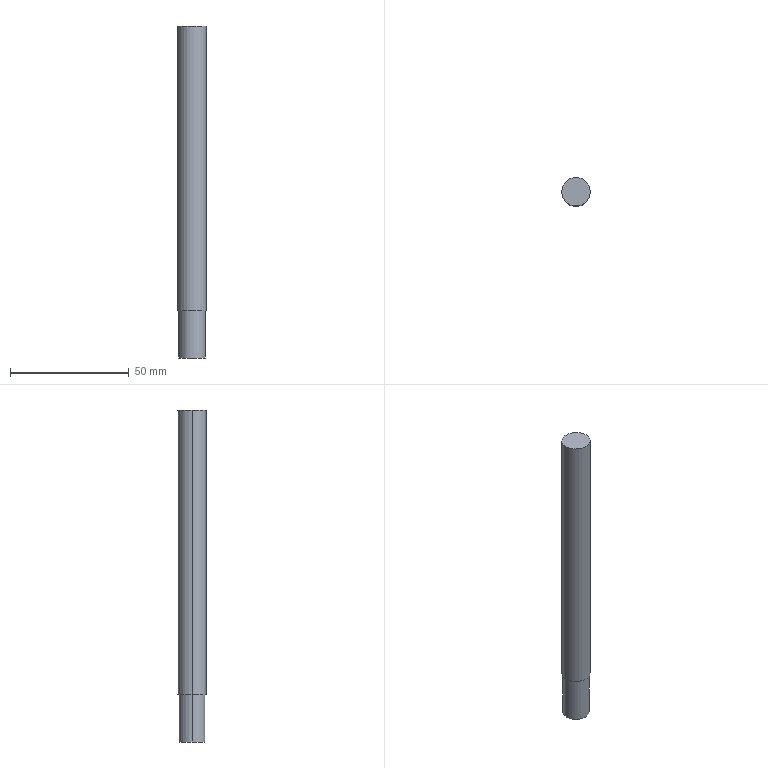Part | SolidWorks | features MirrorStock 1 | 1 solid | 7 faces | box 12 x 12 x 140 mm | volume 15472 mm3 | cylinder 4 | plane 3 | commonest cylinder face diameters 11 x2 12 x2
STEP:
#1=CARTESIAN_POINT('',(-5.5,0.,-50.));
#2=VERTEX_POINT('',#1);
#3=CARTESIAN_POINT('',(5.5,0.,-50.));
#4=VERTEX_POINT('',#3);
#5=CARTESIAN_POINT('',(0.,0.,-50.));
#6=DIRECTION('',(0.,0.,1.));
#7=DIRECTION('',(1.,0.,0.));
#8=AXIS2_PLACEMENT_3D('',#5,#6,#7);
#9=CIRCLE('',#8,5.5);
#10=EDGE_CURVE('',#2,#4,#9,.T.);
#11=ORIENTED_EDGE('',*,*,#10,.F.);
#12=CARTESIAN_POINT('',(-5.5,0.,-70.));
#13=VERTEX_POINT('',#12);
#14=CARTESIAN_POINT('',(-5.5,0.,-50.));
#15=DIRECTION('',(0.,0.,-1.));
#16=VECTOR('',#15,1000.);
#17=LINE('',#14,#16);
#18=EDGE_CURVE('',#2,#13,#17,.T.);
#19=ORIENTED_EDGE('',*,*,#18,.T.);
#20=CARTESIAN_POINT('',(5.5,0.,-70.));
#21=VERTEX_POINT('',#20);
#22=CARTESIAN_POINT('',(0.,0.,-70.));
#23=DIRECTION('',(0.,0.,1.));
#24=DIRECTION('',(1.,0.,0.));
#25=AXIS2_PLACEMENT_3D('',#22,#23,#24);
#26=CIRCLE('',#25,5.5);
#27=EDGE_CURVE('',#13,#21,#26,.T.);
#28=ORIENTED_EDGE('',*,*,#27,.T.);
#29=CARTESIAN_POINT('',(5.5,0.,-50.));
#30=DIRECTION('',(0.,0.,-1.));
#31=VECTOR('',#30,1000.);
#32=LINE('',#29,#31);
#33=EDGE_CURVE('',#4,#21,#32,.T.);
#34=ORIENTED_EDGE('',*,*,#33,.F.);
#35=EDGE_LOOP('',(#11,#19,#28,#34));
#36=FACE_OUTER_BOUND('',#35,.T.);
#37=CARTESIAN_POINT('',(0.,0.,-50.));
#38=DIRECTION('',(0.,0.,-1.));
#39=DIRECTION('',(1.,0.,0.));
#40=AXIS2_PLACEMENT_3D('',#37,#38,#39);
#41=CYLINDRICAL_SURFACE('',#40,5.5);
#42=ADVANCED_FACE('',(#36),#41,.T.);
#43=CARTESIAN_POINT('',(-6.,0.,-50.));
#44=VERTEX_POINT('',#43);
#45=CARTESIAN_POINT('',(6.,0.,-50.));
#46=VERTEX_POINT('',#45);
#47=CARTESIAN_POINT('',(0.,0.,-50.));
#48=DIRECTION('',(0.,0.,1.));
#49=DIRECTION('',(1.,0.,0.));
#50=AXIS2_PLACEMENT_3D('',#47,#48,#49);
#51=CIRCLE('',#50,6.);
#52=EDGE_CURVE('',#44,#46,#51,.T.);
#53=ORIENTED_EDGE('',*,*,#52,.T.);
#54=CARTESIAN_POINT('',(6.,0.,70.));
#55=VERTEX_POINT('',#54);
#56=CARTESIAN_POINT('',(6.,0.,-70.));
#57=DIRECTION('',(0.,0.,1.));
#58=VECTOR('',#57,1000.);
#59=LINE('',#56,#58);
#60=EDGE_CURVE('',#46,#55,#59,.T.);
#61=ORIENTED_EDGE('',*,*,#60,.T.);
#62=CARTESIAN_POINT('',(-6.,0.,70.));
#63=VERTEX_POINT('',#62);
#64=CARTESIAN_POINT('',(0.,0.,70.));
#65=DIRECTION('',(0.,0.,1.));
#66=DIRECTION('',(1.,0.,0.));
#67=AXIS2_PLACEMENT_3D('',#64,#65,#66);
#68=CIRCLE('',#67,6.);
#69=EDGE_CURVE('',#63,#55,#68,.T.);
#70=ORIENTED_EDGE('',*,*,#69,.F.);
#71=CARTESIAN_POINT('',(-6.,0.,-70.));
#72=DIRECTION('',(0.,0.,1.));
#73=VECTOR('',#72,1000.);
#74=LINE('',#71,#73);
#75=EDGE_CURVE('',#44,#63,#74,.T.);
#76=ORIENTED_EDGE('',*,*,#75,.F.);
#77=EDGE_LOOP('',(#53,#61,#70,#76));
#78=FACE_OUTER_BOUND('',#77,.T.);
#79=CARTESIAN_POINT('',(0.,0.,-70.));
#80=DIRECTION('',(0.,0.,1.));
#81=DIRECTION('',(-1.,0.,0.));
#82=AXIS2_PLACEMENT_3D('',#79,#80,#81);
#83=CYLINDRICAL_SURFACE('',#82,6.);
#84=ADVANCED_FACE('',(#78),#83,.T.);
#85=ORIENTED_EDGE('',*,*,#60,.F.);
#86=CARTESIAN_POINT('',(0.,0.,-50.));
#87=DIRECTION('',(0.,0.,1.));
#88=DIRECTION('',(1.,0.,0.));
#89=AXIS2_PLACEMENT_3D('',#86,#87,#88);
#90=CIRCLE('',#89,6.);
#91=EDGE_CURVE('',#46,#44,#90,.T.);
#92=ORIENTED_EDGE('',*,*,#91,.T.);
#93=ORIENTED_EDGE('',*,*,#75,.T.);
#94=CARTESIAN_POINT('',(0.,0.,70.));
#95=DIRECTION('',(0.,0.,1.));
#96=DIRECTION('',(1.,0.,0.));
#97=AXIS2_PLACEMENT_3D('',#94,#95,#96);
#98=CIRCLE('',#97,6.);
#99=EDGE_CURVE('',#55,#63,#98,.T.);
#100=ORIENTED_EDGE('',*,*,#99,.F.);
#101=EDGE_LOOP('',(#85,#92,#93,#100));
#102=FACE_OUTER_BOUND('',#101,.T.);
#103=CARTESIAN_POINT('',(0.,0.,-70.));
#104=DIRECTION('',(0.,0.,1.));
#105=DIRECTION('',(-1.,0.,0.));
#106=AXIS2_PLACEMENT_3D('',#103,#104,#105);
#107=CYLINDRICAL_SURFACE('',#106,6.);
#108=ADVANCED_FACE('',(#102),#107,.T.);
#109=ORIENTED_EDGE('',*,*,#69,.T.);
#110=ORIENTED_EDGE('',*,*,#99,.T.);
#111=EDGE_LOOP('',(#109,#110));
#112=FACE_OUTER_BOUND('',#111,.T.);
#113=CARTESIAN_POINT('',(0.,0.,70.));
#114=DIRECTION('',(0.,0.,-1.));
#115=DIRECTION('',(1.,0.,0.));
#116=AXIS2_PLACEMENT_3D('',#113,#114,#115);
#117=PLANE('',#116);
#118=ADVANCED_FACE('',(#112),#117,.F.);
#119=CARTESIAN_POINT('',(0.,0.,-50.));
#120=DIRECTION('',(0.,0.,1.));
#121=DIRECTION('',(1.,0.,0.));
#122=AXIS2_PLACEMENT_3D('',#119,#120,#121);
#123=CIRCLE('',#122,5.5);
#124=EDGE_CURVE('',#4,#2,#123,.T.);
#125=ORIENTED_EDGE('',*,*,#124,.T.);
#126=ORIENTED_EDGE('',*,*,#10,.T.);
#127=EDGE_LOOP('',(#125,#126));
#128=FACE_BOUND('',#127,.T.);
#129=ORIENTED_EDGE('',*,*,#52,.F.);
#130=ORIENTED_EDGE('',*,*,#91,.F.);
#131=EDGE_LOOP('',(#129,#130));
#132=FACE_OUTER_BOUND('',#131,.T.);
#133=CARTESIAN_POINT('',(0.,0.,-50.));
#134=DIRECTION('',(0.,0.,-1.));
#135=DIRECTION('',(1.,0.,0.));
#136=AXIS2_PLACEMENT_3D('',#133,#134,#135);
#137=PLANE('',#136);
#138=ADVANCED_FACE('',(#128,#132),#137,.T.);
#139=ORIENTED_EDGE('',*,*,#18,.F.);
#140=ORIENTED_EDGE('',*,*,#124,.F.);
#141=ORIENTED_EDGE('',*,*,#33,.T.);
#142=CARTESIAN_POINT('',(0.,0.,-70.));
#143=DIRECTION('',(0.,0.,1.));
#144=DIRECTION('',(1.,0.,0.));
#145=AXIS2_PLACEMENT_3D('',#142,#143,#144);
#146=CIRCLE('',#145,5.5);
#147=EDGE_CURVE('',#21,#13,#146,.T.);
#148=ORIENTED_EDGE('',*,*,#147,.T.);
#149=EDGE_LOOP('',(#139,#140,#141,#148));
#150=FACE_OUTER_BOUND('',#149,.T.);
#151=CARTESIAN_POINT('',(0.,0.,-50.));
#152=DIRECTION('',(0.,0.,-1.));
#153=DIRECTION('',(1.,0.,0.));
#154=AXIS2_PLACEMENT_3D('',#151,#152,#153);
#155=CYLINDRICAL_SURFACE('',#154,5.5);
#156=ADVANCED_FACE('',(#150),#155,.T.);
#157=ORIENTED_EDGE('',*,*,#147,.F.);
#158=ORIENTED_EDGE('',*,*,#27,.F.);
#159=EDGE_LOOP('',(#157,#158));
#160=FACE_OUTER_BOUND('',#159,.T.);
#161=CARTESIAN_POINT('',(0.,0.,-70.));
#162=DIRECTION('',(0.,0.,-1.));
#163=DIRECTION('',(1.,0.,0.));
#164=AXIS2_PLACEMENT_3D('',#161,#162,#163);
#165=PLANE('',#164);
#166=ADVANCED_FACE('',(#160),#165,.T.);
#167=CLOSED_SHELL('',(#42,#84,#108,#118,#138,#156,#166));
#168=MANIFOLD_SOLID_BREP('',#167);
#169=CARTESIAN_POINT('',(0.,0.,0.));
#170=DIRECTION('',(0.,0.,1.));
#171=DIRECTION('',(1.,0.,0.));
#172=AXIS2_PLACEMENT_3D('',#169,#170,#171);
#173=(LENGTH_UNIT()NAMED_UNIT(*)SI_UNIT(.MILLI.,.METRE.));
#174=UNCERTAINTY_MEASURE_WITH_UNIT(LENGTH_MEASURE(0.00001),#173,'','');
#175=(NAMED_UNIT(*)PLANE_ANGLE_UNIT()SI_UNIT($,.RADIAN.));
#176=(NAMED_UNIT(*)SI_UNIT($,.STERADIAN.)SOLID_ANGLE_UNIT());
#177=(GEOMETRIC_REPRESENTATION_CONTEXT(3)GLOBAL_UNCERTAINTY_ASSIGNED_CONTEXT((#174))GLOBAL_UNIT_ASSIGNED_CONTEXT((#173,#175,#176))REPRESENTATION_CONTEXT('',''));
#178=ADVANCED_BREP_SHAPE_REPRESENTATION('',(#168,#172),#177);